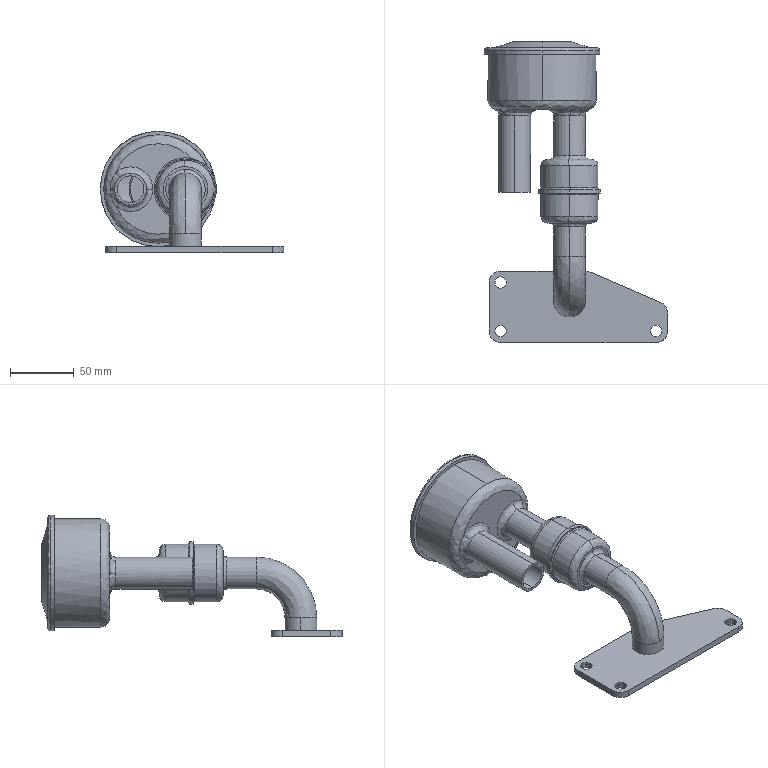Part | SolidWorks | features BaseBody 1 | 1 solid | 130 faces | box 143.75 x 235.871 x 95.25 mm | volume 181252 mm3 | cylinder 52 | spline 45 | plane 29 | cone 4 | commonest cylinder face diameters 9 x12 21 x8 25 x8 14 x5 18 x5 45 x4